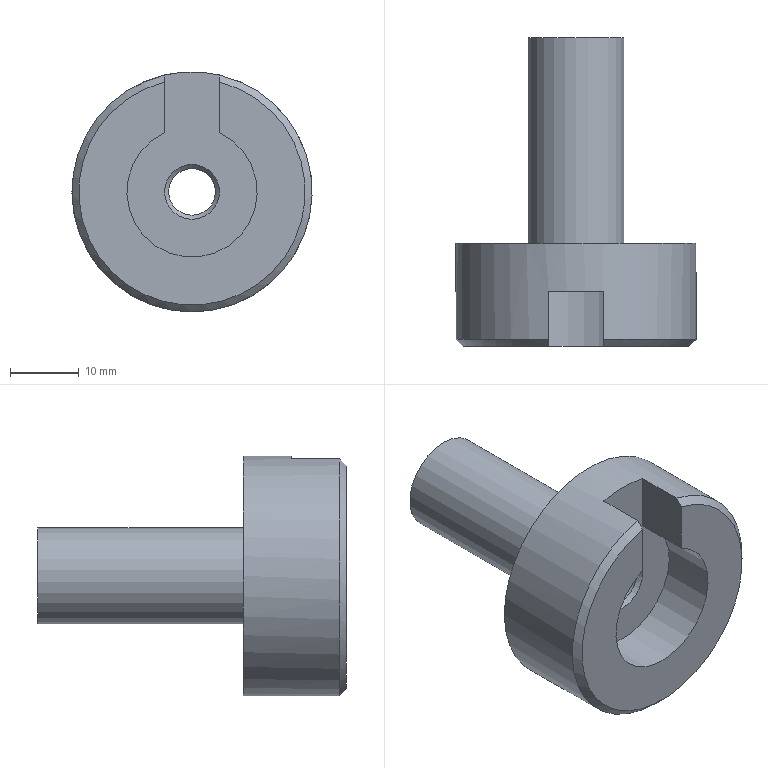Part | STEP file | 冲床-300配套压波_id602_x_t | 1 solid | 12 faces | box 35 x 45 x 35 mm | volume 14863 mm3 | plane 6 | cylinder 4 | cone 2 | commonest cylinder face diameters 6.8 x1 14 x1 19 x1 35 x1
STEP:
#1=CARTESIAN_POINT('',(1388.,127.,88.7));
#2=VERTEX_POINT('',#1);
#3=CARTESIAN_POINT('',(1396.,127.,88.7));
#4=VERTEX_POINT('',#3);
#5=CARTESIAN_POINT('',(1392.,127.,80.083));
#6=DIRECTION('',(0.,-1.,0.));
#7=DIRECTION('',(0.,0.,-1.));
#8=AXIS2_PLACEMENT_3D('',#5,#6,#7);
#9=CIRCLE('',#8,9.5);
#10=EDGE_CURVE('',#2,#4,#9,.T.);
#11=ORIENTED_EDGE('',*,*,#10,.T.);
#12=CARTESIAN_POINT('',(1396.,135.,88.7));
#13=VERTEX_POINT('',#12);
#14=CARTESIAN_POINT('',(1396.,140.,88.7));
#15=DIRECTION('',(0.,1.,0.));
#16=VECTOR('',#15,1.);
#17=LINE('',#14,#16);
#18=EDGE_CURVE('',#4,#13,#17,.T.);
#19=ORIENTED_EDGE('',*,*,#18,.T.);
#20=CARTESIAN_POINT('',(1388.,135.,88.7));
#21=VERTEX_POINT('',#20);
#22=CARTESIAN_POINT('',(1392.,135.,80.083));
#23=DIRECTION('',(0.,1.,0.));
#24=DIRECTION('',(0.,0.,-1.));
#25=AXIS2_PLACEMENT_3D('',#22,#23,#24);
#26=CIRCLE('',#25,9.5);
#27=EDGE_CURVE('',#13,#21,#26,.T.);
#28=ORIENTED_EDGE('',*,*,#27,.T.);
#29=CARTESIAN_POINT('',(1388.,140.,88.7));
#30=DIRECTION('',(0.,-1.,0.));
#31=VECTOR('',#30,1.);
#32=LINE('',#29,#31);
#33=EDGE_CURVE('',#21,#2,#32,.T.);
#34=ORIENTED_EDGE('',*,*,#33,.T.);
#35=EDGE_LOOP('',(#11,#19,#28,#34));
#36=FACE_OUTER_BOUND('',#35,.T.);
#37=CARTESIAN_POINT('',(1392.,140.,80.083));
#38=DIRECTION('',(0.,-1.,0.));
#39=DIRECTION('',(-1.,0.,0.));
#40=AXIS2_PLACEMENT_3D('',#37,#38,#39);
#41=CYLINDRICAL_SURFACE('',#40,9.5);
#42=ADVANCED_FACE('',(#36),#41,.F.);
#43=CARTESIAN_POINT('',(1374.5,142.,80.083));
#44=VERTEX_POINT('',#43);
#45=CARTESIAN_POINT('',(1392.,142.,80.083));
#46=DIRECTION('',(0.,1.,0.));
#47=DIRECTION('',(-1.,0.,0.));
#48=AXIS2_PLACEMENT_3D('',#45,#46,#47);
#49=CIRCLE('',#48,17.5);
#50=EDGE_CURVE('',#44,#44,#49,.T.);
#51=ORIENTED_EDGE('',*,*,#50,.F.);
#52=EDGE_LOOP('',(#51));
#53=FACE_BOUND('',#52,.T.);
#54=CARTESIAN_POINT('',(1388.,135.,97.12));
#55=VERTEX_POINT('',#54);
#56=CARTESIAN_POINT('',(1388.,128.,97.12));
#57=VERTEX_POINT('',#56);
#58=CARTESIAN_POINT('',(1388.,142.,97.12));
#59=DIRECTION('',(0.,-1.,0.));
#60=VECTOR('',#59,1.);
#61=LINE('',#58,#60);
#62=EDGE_CURVE('',#55,#57,#61,.T.);
#63=ORIENTED_EDGE('',*,*,#62,.F.);
#64=CARTESIAN_POINT('',(1396.,135.,97.12));
#65=VERTEX_POINT('',#64);
#66=CARTESIAN_POINT('',(1392.,135.,80.083));
#67=DIRECTION('',(0.,1.,0.));
#68=DIRECTION('',(0.,0.,1.));
#69=AXIS2_PLACEMENT_3D('',#66,#67,#68);
#70=CIRCLE('',#69,17.5);
#71=EDGE_CURVE('',#55,#65,#70,.T.);
#72=ORIENTED_EDGE('',*,*,#71,.T.);
#73=CARTESIAN_POINT('',(1396.,128.,97.12));
#74=VERTEX_POINT('',#73);
#75=CARTESIAN_POINT('',(1396.,142.,97.12));
#76=DIRECTION('',(0.,1.,0.));
#77=VECTOR('',#76,1.);
#78=LINE('',#75,#77);
#79=EDGE_CURVE('',#74,#65,#78,.T.);
#80=ORIENTED_EDGE('',*,*,#79,.F.);
#81=CARTESIAN_POINT('',(1392.,128.,80.083));
#82=DIRECTION('',(0.,1.,0.));
#83=DIRECTION('',(0.,0.,-1.));
#84=AXIS2_PLACEMENT_3D('',#81,#82,#83);
#85=CIRCLE('',#84,17.5);
#86=EDGE_CURVE('',#74,#57,#85,.T.);
#87=ORIENTED_EDGE('',*,*,#86,.T.);
#88=EDGE_LOOP('',(#63,#72,#80,#87));
#89=FACE_BOUND('',#88,.T.);
#90=CARTESIAN_POINT('',(1392.,142.,80.083));
#91=DIRECTION('',(0.,-1.,0.));
#92=DIRECTION('',(0.,0.,1.));
#93=AXIS2_PLACEMENT_3D('',#90,#91,#92);
#94=CYLINDRICAL_SURFACE('',#93,17.5);
#95=ADVANCED_FACE('',(#53,#89),#94,.T.);
#96=CARTESIAN_POINT('',(1396.,127.,96.091));
#97=VERTEX_POINT('',#96);
#98=CARTESIAN_POINT('',(1396.,127.,80.083));
#99=DIRECTION('',(0.,0.,-1.));
#100=VECTOR('',#99,1.);
#101=LINE('',#98,#100);
#102=EDGE_CURVE('',#97,#4,#101,.T.);
#103=ORIENTED_EDGE('',*,*,#102,.T.);
#104=ORIENTED_EDGE('',*,*,#10,.F.);
#105=CARTESIAN_POINT('',(1388.,127.,96.091));
#106=VERTEX_POINT('',#105);
#107=CARTESIAN_POINT('',(1388.,127.,80.083));
#108=DIRECTION('',(0.,0.,-1.));
#109=VECTOR('',#108,1.);
#110=LINE('',#107,#109);
#111=EDGE_CURVE('',#106,#2,#110,.T.);
#112=ORIENTED_EDGE('',*,*,#111,.F.);
#113=CARTESIAN_POINT('',(1392.,127.,80.083));
#114=DIRECTION('',(0.,-1.,0.));
#115=DIRECTION('',(0.,0.,-1.));
#116=AXIS2_PLACEMENT_3D('',#113,#114,#115);
#117=CIRCLE('',#116,16.5);
#118=EDGE_CURVE('',#106,#97,#117,.T.);
#119=ORIENTED_EDGE('',*,*,#118,.T.);
#120=EDGE_LOOP('',(#103,#104,#112,#119));
#121=FACE_OUTER_BOUND('',#120,.T.);
#122=CARTESIAN_POINT('',(1392.,127.,80.083));
#123=DIRECTION('',(0.,1.,0.));
#124=DIRECTION('',(0.,0.,-1.));
#125=AXIS2_PLACEMENT_3D('',#122,#123,#124);
#126=PLANE('',#125);
#127=ADVANCED_FACE('',(#121),#126,.F.);
#128=ORIENTED_EDGE('',*,*,#27,.F.);
#129=CARTESIAN_POINT('',(1396.,135.,100.583));
#130=DIRECTION('',(0.,0.,1.));
#131=VECTOR('',#130,1.);
#132=LINE('',#129,#131);
#133=EDGE_CURVE('',#13,#65,#132,.T.);
#134=ORIENTED_EDGE('',*,*,#133,.T.);
#135=ORIENTED_EDGE('',*,*,#71,.F.);
#136=CARTESIAN_POINT('',(1388.,135.,100.583));
#137=DIRECTION('',(0.,0.,1.));
#138=VECTOR('',#137,1.);
#139=LINE('',#136,#138);
#140=EDGE_CURVE('',#21,#55,#139,.T.);
#141=ORIENTED_EDGE('',*,*,#140,.F.);
#142=EDGE_LOOP('',(#128,#134,#135,#141));
#143=FACE_BOUND('',#142,.T.);
#144=CARTESIAN_POINT('',(1392.,135.,76.083));
#145=VERTEX_POINT('',#144);
#146=CARTESIAN_POINT('',(1392.,135.,80.083));
#147=DIRECTION('',(0.,1.,0.));
#148=DIRECTION('',(0.,0.,-1.));
#149=AXIS2_PLACEMENT_3D('',#146,#147,#148);
#150=CIRCLE('',#149,4.);
#151=EDGE_CURVE('',#145,#145,#150,.T.);
#152=ORIENTED_EDGE('',*,*,#151,.T.);
#153=EDGE_LOOP('',(#152));
#154=FACE_BOUND('',#153,.T.);
#155=CARTESIAN_POINT('',(1392.,135.,80.083));
#156=DIRECTION('',(0.,1.,0.));
#157=DIRECTION('',(0.,0.,-1.));
#158=AXIS2_PLACEMENT_3D('',#155,#156,#157);
#159=PLANE('',#158);
#160=ADVANCED_FACE('',(#143,#154),#159,.F.);
#161=CARTESIAN_POINT('',(1392.,142.,87.083));
#162=VERTEX_POINT('',#161);
#163=CARTESIAN_POINT('',(1392.,142.,80.083));
#164=DIRECTION('',(0.,1.,0.));
#165=DIRECTION('',(0.,0.,1.));
#166=AXIS2_PLACEMENT_3D('',#163,#164,#165);
#167=CIRCLE('',#166,7.);
#168=EDGE_CURVE('',#162,#162,#167,.T.);
#169=ORIENTED_EDGE('',*,*,#168,.F.);
#170=EDGE_LOOP('',(#169));
#171=FACE_BOUND('',#170,.T.);
#172=ORIENTED_EDGE('',*,*,#50,.T.);
#173=EDGE_LOOP('',(#172));
#174=FACE_BOUND('',#173,.T.);
#175=CARTESIAN_POINT('',(1392.,142.,80.083));
#176=DIRECTION('',(0.,1.,0.));
#177=DIRECTION('',(0.,0.,-1.));
#178=AXIS2_PLACEMENT_3D('',#175,#176,#177);
#179=PLANE('',#178);
#180=ADVANCED_FACE('',(#171,#174),#179,.T.);
#181=CARTESIAN_POINT('',(1392.,135.6,76.683));
#182=VERTEX_POINT('',#181);
#183=CARTESIAN_POINT('',(1392.,135.6,80.083));
#184=DIRECTION('',(0.,-1.,0.));
#185=DIRECTION('',(0.,0.,-1.));
#186=AXIS2_PLACEMENT_3D('',#183,#184,#185);
#187=CIRCLE('',#186,3.4);
#188=EDGE_CURVE('',#182,#182,#187,.T.);
#189=ORIENTED_EDGE('',*,*,#188,.T.);
#190=EDGE_LOOP('',(#189));
#191=FACE_BOUND('',#190,.T.);
#192=CARTESIAN_POINT('',(1392.,172.,83.483));
#193=VERTEX_POINT('',#192);
#194=CARTESIAN_POINT('',(1392.,172.,80.083));
#195=DIRECTION('',(0.,1.,0.));
#196=DIRECTION('',(0.,0.,1.));
#197=AXIS2_PLACEMENT_3D('',#194,#195,#196);
#198=CIRCLE('',#197,3.4);
#199=EDGE_CURVE('',#193,#193,#198,.T.);
#200=ORIENTED_EDGE('',*,*,#199,.T.);
#201=EDGE_LOOP('',(#200));
#202=FACE_BOUND('',#201,.T.);
#203=CARTESIAN_POINT('',(1392.,135.,80.083));
#204=DIRECTION('',(0.,1.,0.));
#205=DIRECTION('',(0.,0.,-1.));
#206=AXIS2_PLACEMENT_3D('',#203,#204,#205);
#207=CYLINDRICAL_SURFACE('',#206,3.4);
#208=ADVANCED_FACE('',(#191,#202),#207,.F.);
#209=ORIENTED_EDGE('',*,*,#188,.F.);
#210=EDGE_LOOP('',(#209));
#211=FACE_BOUND('',#210,.T.);
#212=ORIENTED_EDGE('',*,*,#151,.F.);
#213=EDGE_LOOP('',(#212));
#214=FACE_BOUND('',#213,.T.);
#215=CARTESIAN_POINT('',(1392.,135.,80.083));
#216=DIRECTION('',(0.,-1.,0.));
#217=DIRECTION('',(0.,0.,1.));
#218=AXIS2_PLACEMENT_3D('',#215,#216,#217);
#219=CONICAL_SURFACE('',#218,4.,45.);
#220=ADVANCED_FACE('',(#211,#214),#219,.F.);
#221=ORIENTED_EDGE('',*,*,#111,.T.);
#222=ORIENTED_EDGE('',*,*,#33,.F.);
#223=ORIENTED_EDGE('',*,*,#140,.T.);
#224=ORIENTED_EDGE('',*,*,#62,.T.);
#225=CARTESIAN_POINT('',(1388.,128.,97.12));
#226=CARTESIAN_POINT('',(1388.,127.666,96.778));
#227=CARTESIAN_POINT('',(1388.,127.333,96.435));
#228=CARTESIAN_POINT('',(1388.,127.,96.091));
#229=B_SPLINE_CURVE_WITH_KNOTS('',3,(#225,#226,#227,#228),.UNSPECIFIED.,.F.,.F.,(4,4),(0.,1.),.UNSPECIFIED.);
#230=EDGE_CURVE('',#57,#106,#229,.T.);
#231=ORIENTED_EDGE('',*,*,#230,.T.);
#232=EDGE_LOOP('',(#221,#222,#223,#224,#231));
#233=FACE_OUTER_BOUND('',#232,.T.);
#234=CARTESIAN_POINT('',(1388.,116.,100.583));
#235=DIRECTION('',(1.,0.,0.));
#236=DIRECTION('',(0.,0.,-1.));
#237=AXIS2_PLACEMENT_3D('',#234,#235,#236);
#238=PLANE('',#237);
#239=ADVANCED_FACE('',(#233),#238,.T.);
#240=ORIENTED_EDGE('',*,*,#79,.T.);
#241=ORIENTED_EDGE('',*,*,#133,.F.);
#242=ORIENTED_EDGE('',*,*,#18,.F.);
#243=ORIENTED_EDGE('',*,*,#102,.F.);
#244=CARTESIAN_POINT('',(1396.,127.,96.091));
#245=CARTESIAN_POINT('',(1396.,127.333,96.435));
#246=CARTESIAN_POINT('',(1396.,127.666,96.778));
#247=CARTESIAN_POINT('',(1396.,128.,97.12));
#248=B_SPLINE_CURVE_WITH_KNOTS('',3,(#244,#245,#246,#247),.UNSPECIFIED.,.F.,.F.,(4,4),(0.,1.),.UNSPECIFIED.);
#249=EDGE_CURVE('',#97,#74,#248,.T.);
#250=ORIENTED_EDGE('',*,*,#249,.T.);
#251=EDGE_LOOP('',(#240,#241,#242,#243,#250));
#252=FACE_OUTER_BOUND('',#251,.T.);
#253=CARTESIAN_POINT('',(1396.,135.,100.583));
#254=DIRECTION('',(-1.,0.,0.));
#255=DIRECTION('',(0.,1.,0.));
#256=AXIS2_PLACEMENT_3D('',#253,#254,#255);
#257=PLANE('',#256);
#258=ADVANCED_FACE('',(#252),#257,.T.);
#259=ORIENTED_EDGE('',*,*,#230,.F.);
#260=ORIENTED_EDGE('',*,*,#86,.F.);
#261=ORIENTED_EDGE('',*,*,#249,.F.);
#262=ORIENTED_EDGE('',*,*,#118,.F.);
#263=EDGE_LOOP('',(#259,#260,#261,#262));
#264=FACE_OUTER_BOUND('',#263,.T.);
#265=CARTESIAN_POINT('',(1392.,128.,80.083));
#266=DIRECTION('',(0.,1.,0.));
#267=DIRECTION('',(0.,0.,-1.));
#268=AXIS2_PLACEMENT_3D('',#265,#266,#267);
#269=CONICAL_SURFACE('',#268,17.5,45.);
#270=ADVANCED_FACE('',(#264),#269,.T.);
#271=CARTESIAN_POINT('',(1392.,172.,87.083));
#272=VERTEX_POINT('',#271);
#273=CARTESIAN_POINT('',(1392.,172.,80.083));
#274=DIRECTION('',(0.,1.,0.));
#275=DIRECTION('',(0.,0.,1.));
#276=AXIS2_PLACEMENT_3D('',#273,#274,#275);
#277=CIRCLE('',#276,7.);
#278=EDGE_CURVE('',#272,#272,#277,.T.);
#279=ORIENTED_EDGE('',*,*,#278,.F.);
#280=EDGE_LOOP('',(#279));
#281=FACE_BOUND('',#280,.T.);
#282=ORIENTED_EDGE('',*,*,#168,.T.);
#283=EDGE_LOOP('',(#282));
#284=FACE_BOUND('',#283,.T.);
#285=CARTESIAN_POINT('',(1392.,172.,80.083));
#286=DIRECTION('',(0.,-1.,0.));
#287=DIRECTION('',(1.,0.,0.));
#288=AXIS2_PLACEMENT_3D('',#285,#286,#287);
#289=CYLINDRICAL_SURFACE('',#288,7.);
#290=ADVANCED_FACE('',(#281,#284),#289,.T.);
#291=ORIENTED_EDGE('',*,*,#278,.T.);
#292=EDGE_LOOP('',(#291));
#293=FACE_BOUND('',#292,.T.);
#294=ORIENTED_EDGE('',*,*,#199,.F.);
#295=EDGE_LOOP('',(#294));
#296=FACE_BOUND('',#295,.T.);
#297=CARTESIAN_POINT('',(1392.,172.,80.083));
#298=DIRECTION('',(0.,1.,0.));
#299=DIRECTION('',(0.,0.,1.));
#300=AXIS2_PLACEMENT_3D('',#297,#298,#299);
#301=PLANE('',#300);
#302=ADVANCED_FACE('',(#293,#296),#301,.T.);
#303=CLOSED_SHELL('',(#42,#95,#127,#160,#180,#208,#220,#239,#258,#270,#290,#302));
#304=MANIFOLD_SOLID_BREP('',#303);
#305=(LENGTH_UNIT()NAMED_UNIT(*)SI_UNIT(.MILLI.,.METRE.));
#306=UNCERTAINTY_MEASURE_WITH_UNIT(LENGTH_MEASURE(0.0508),#305,'','');
#307=(NAMED_UNIT(*)PLANE_ANGLE_UNIT()SI_UNIT($,.RADIAN.));
#308=PLANE_ANGLE_MEASURE_WITH_UNIT(PLANE_ANGLE_MEASURE(0.01745),#307);
#309=DIMENSIONAL_EXPONENTS(0.,0.,0.,0.,0.,0.,0.);
#310=(CONVERSION_BASED_UNIT('DEGREE',#308)NAMED_UNIT(#309)PLANE_ANGLE_UNIT());
#311=(NAMED_UNIT(*)SI_UNIT($,.STERADIAN.)SOLID_ANGLE_UNIT());
#312=(GEOMETRIC_REPRESENTATION_CONTEXT(3)GLOBAL_UNCERTAINTY_ASSIGNED_CONTEXT((#306))GLOBAL_UNIT_ASSIGNED_CONTEXT((#305,#310,#311))REPRESENTATION_CONTEXT('',''));
#313=ADVANCED_BREP_SHAPE_REPRESENTATION('',(#304),#312);